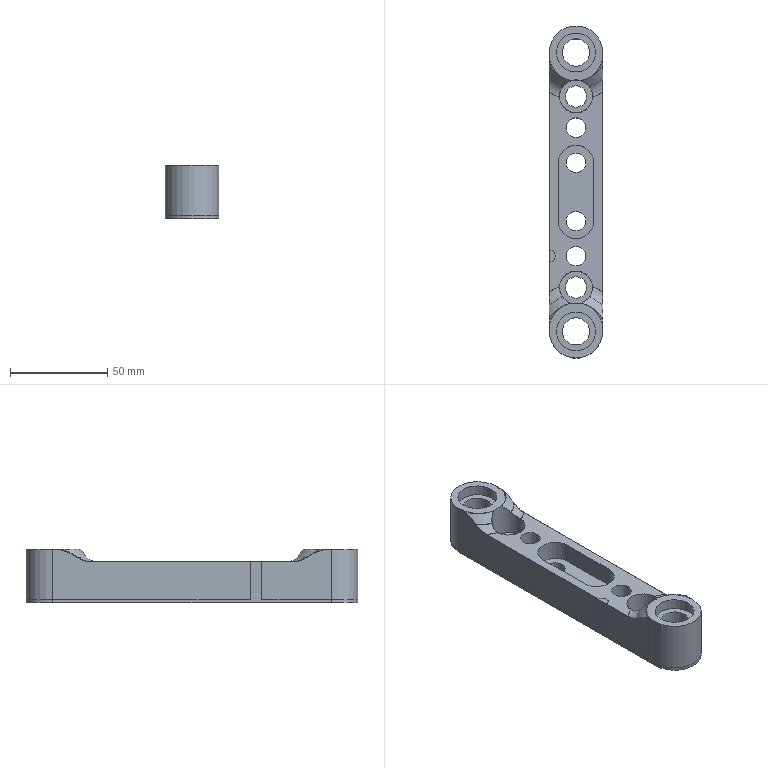NC program | NX | posted with a generic post | part box 27.4 x 170.48 x 27.5 mm
Lines 1 to 120 of 1859:
N10 G17 G21 G94 G90
(DRILLING_4 , TOOL : D8点钻)
N12 T02 M6
N14 G54
N16 G17 G0 G90 X-71.54 Y0. B0. C0. S2000 M3
N18 G43 Z30. H2
N20 G94 G81 G98 Z-1.5 F200. R3.
N22 X-49.
N24 X49.
N26 X71.54
N28 G80
N30 G0 X71.54 Y0. Z30.
(DRILLING_5_COPY_1_COPY , TOOL : D8点钻)
N32 X-33.
N34 G83 Z-1.5 F200. Q1.5 R3.
N36 X-15.
N38 X15.
N40 X33.
N42 G80
N44 G0 X33. Y0. Z30.
N46 M5
(DRILLING_5_COPY_1 , TOOL : Z8.5)
N48 T17 M6
N50 G54
N52 G17 G0 G90 X-33. Y0. B0. C0. S2000 M3
N54 G43 Z30. H17
N56 G94 G83 G98 Z-6. F200. Q2. R3.
N58 X-15.
N60 X15.
N62 X33.
N64 G80
N66 G0 X33. Y0. Z30.
(DRILLING_5 , TOOL : Z8.5)
N68 X-71.54
N70 G83 Z-13. F200. Q2. R3.
N72 X71.54
N74 G80
N76 G0 X71.54 Y0. Z30.
(DRILLING_5_COPY , TOOL : Z8.5)
N78 X-49.
N80 G83 Z-25. F200. Q2. R3.
N82 X49.
N84 G80
N86 G0 X49. Y0. Z30.
N88 M5
(PLANAR_MILL_7 , TOOL : D8点钻)
N90 T02 M6
N92 G54
N94 G17 G0 G90 X-73.54 Y-0.917 B0. C0. S3000 M3
N96 G43 Z30. H2
N98 Z0.
N100 G94 G1 Z-2. F600.
N102 Y-2.2
N104 G3 X-71.54 Y-4.2 R2.
N106 X-67.34 Y0. R4.2
N108 X-71.54 Y-4.2 R-4.2
N110 X-69.54 Y-2.2 R2.
N112 G1 Y-0.917
N114 Z0.
N116 G0 Z30.
N118 X-47.705 Y1.101
N120 Z0.
N122 G1 Z-2.
N124 X-47. Y1.7
N126 G3 X-49. Y3.7 R2.
N128 X-52.7 Y0. R3.7
N130 X-49. Y3.7 R-3.7
N132 X-51. Y1.7 R2.
N134 G1 X-50.295 Y1.101
N136 Z0.
N138 G0 Z30.
N140 X50.295
N142 Z0.
N144 G1 Z-2.
N146 X51. Y1.7
N148 G3 X49. Y3.7 R2.
N150 X45.3 Y0. R3.7
N152 X49. Y3.7 R-3.7
N154 X47. Y1.7 R2.
N156 G1 X47.705 Y1.101
N158 Z0.
N160 G0 Z30.
N162 X69.54 Y-0.917
N164 Z0.
N166 G1 Z-2.
N168 Y-2.2
N170 G3 X71.54 Y-4.2 R2.
N172 X75.74 Y0. R4.2
N174 X71.54 Y-4.2 R-4.2
N176 X73.54 Y-2.2 R2.
N178 G1 Y-0.917
N180 Z0.
N182 G0 Z30.
N184 M5
(DRILLING_5_COPY_COPY , TOOL : M10X1.5)
N186 T18 M6
N188 G54
N190 G17 G0 G90 X-49. Y0. B0. C0. S300 M3
N192 G43 Z30. H18
N194 G84 G94 G98 Z-10. F450. R3.
N196 X49.
N198 G80
N200 G0 X49. Y0. Z30.
N202 M5